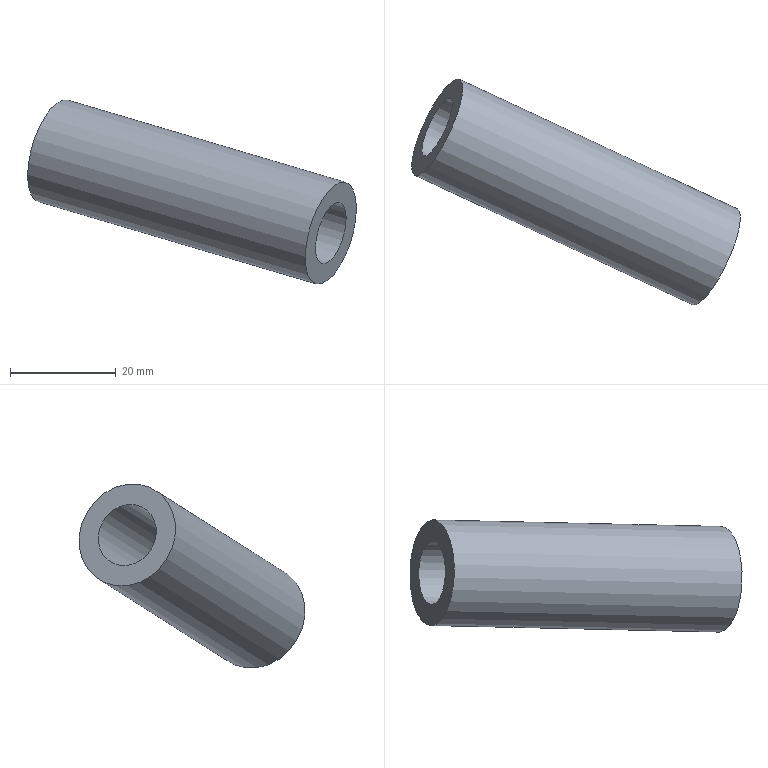Part | NX | features solid 2 | 1 solid | 4 faces | box 62.193 x 42.751 x 34.848 mm | volume 12064 mm3 | cylinder 2 | plane 2 | commonest cylinder face diameters 12 x1 20 x1
STEP:
#1=CARTESIAN_POINT('',(-896.209,778.382,-91.518));
#2=VERTEX_POINT('',#1);
#3=CARTESIAN_POINT('',(-891.983,787.445,-91.518));
#4=DIRECTION('',(-0.8754,0.4082,0.2588));
#5=DIRECTION('',(-0.4226,-0.9063,-0.000000003));
#6=AXIS2_PLACEMENT_3D('',#3,#4,#5);
#7=CIRCLE('',#6,10.);
#8=EDGE_CURVE('',#2,#2,#7,.F.);
#9=ORIENTED_EDGE('',*,*,#8,.T.);
#10=EDGE_LOOP('',(#9));
#11=FACE_BOUND('',#10,.T.);
#12=CARTESIAN_POINT('',(-843.684,753.889,-107.047));
#13=VERTEX_POINT('',#12);
#14=CARTESIAN_POINT('',(-839.458,762.952,-107.047));
#15=DIRECTION('',(-0.8754,0.4082,0.2588));
#16=DIRECTION('',(-0.4226,-0.9063,-0.000000003));
#17=AXIS2_PLACEMENT_3D('',#14,#15,#16);
#18=CIRCLE('',#17,10.);
#19=EDGE_CURVE('',#13,#13,#18,.F.);
#20=ORIENTED_EDGE('',*,*,#19,.F.);
#21=EDGE_LOOP('',(#20));
#22=FACE_BOUND('',#21,.T.);
#23=CARTESIAN_POINT('',(-839.458,762.952,-107.047));
#24=DIRECTION('',(-0.8754,0.4082,0.2588));
#25=DIRECTION('',(-0.4226,-0.9063,-0.000000003));
#26=AXIS2_PLACEMENT_3D('',#23,#24,#25);
#27=CYLINDRICAL_SURFACE('',#26,10.);
#28=ADVANCED_FACE('',(#11,#22),#27,.T.);
#29=ORIENTED_EDGE('',*,*,#19,.T.);
#30=EDGE_LOOP('',(#29));
#31=FACE_BOUND('',#30,.T.);
#32=CARTESIAN_POINT('',(-841.993,757.514,-107.047));
#33=VERTEX_POINT('',#32);
#34=CARTESIAN_POINT('',(-839.458,762.952,-107.047));
#35=DIRECTION('',(0.8754,-0.4082,-0.2588));
#36=DIRECTION('',(-0.4226,-0.9063,-0.000000003));
#37=AXIS2_PLACEMENT_3D('',#34,#35,#36);
#38=CIRCLE('',#37,6.);
#39=EDGE_CURVE('',#33,#33,#38,.T.);
#40=ORIENTED_EDGE('',*,*,#39,.F.);
#41=EDGE_LOOP('',(#40));
#42=FACE_BOUND('',#41,.T.);
#43=CARTESIAN_POINT('',(-839.458,762.952,-107.047));
#44=DIRECTION('',(-0.8754,0.4082,0.2588));
#45=DIRECTION('',(-0.4226,-0.9063,-0.000000003));
#46=AXIS2_PLACEMENT_3D('',#43,#44,#45);
#47=PLANE('',#46);
#48=ADVANCED_FACE('',(#31,#42),#47,.F.);
#49=ORIENTED_EDGE('',*,*,#8,.F.);
#50=EDGE_LOOP('',(#49));
#51=FACE_BOUND('',#50,.T.);
#52=CARTESIAN_POINT('',(-894.519,782.007,-91.518));
#53=VERTEX_POINT('',#52);
#54=CARTESIAN_POINT('',(-891.983,787.445,-91.518));
#55=DIRECTION('',(-0.8754,0.4082,0.2588));
#56=DIRECTION('',(-0.4226,-0.9063,-0.000000003));
#57=AXIS2_PLACEMENT_3D('',#54,#55,#56);
#58=CIRCLE('',#57,6.);
#59=EDGE_CURVE('',#53,#53,#58,.F.);
#60=ORIENTED_EDGE('',*,*,#59,.T.);
#61=EDGE_LOOP('',(#60));
#62=FACE_BOUND('',#61,.T.);
#63=CARTESIAN_POINT('',(-891.983,787.445,-91.518));
#64=DIRECTION('',(-0.8754,0.4082,0.2588));
#65=DIRECTION('',(-0.4226,-0.9063,-0.000000003));
#66=AXIS2_PLACEMENT_3D('',#63,#64,#65);
#67=PLANE('',#66);
#68=ADVANCED_FACE('',(#51,#62),#67,.T.);
#69=ORIENTED_EDGE('',*,*,#59,.F.);
#70=EDGE_LOOP('',(#69));
#71=FACE_BOUND('',#70,.T.);
#72=ORIENTED_EDGE('',*,*,#39,.T.);
#73=EDGE_LOOP('',(#72));
#74=FACE_BOUND('',#73,.T.);
#75=CARTESIAN_POINT('',(-839.458,762.952,-107.047));
#76=DIRECTION('',(-0.8754,0.4082,0.2588));
#77=DIRECTION('',(-0.4226,-0.9063,-0.000000003));
#78=AXIS2_PLACEMENT_3D('',#75,#76,#77);
#79=CYLINDRICAL_SURFACE('',#78,6.);
#80=ADVANCED_FACE('',(#71,#74),#79,.F.);
#81=CLOSED_SHELL('',(#28,#48,#68,#80));
#82=MANIFOLD_SOLID_BREP('',#81);
#83=(LENGTH_UNIT()NAMED_UNIT(*)SI_UNIT(.MILLI.,.METRE.));
#84=UNCERTAINTY_MEASURE_WITH_UNIT(LENGTH_MEASURE(0.00001),#83,'','');
#85=(NAMED_UNIT(*)PLANE_ANGLE_UNIT()SI_UNIT($,.RADIAN.));
#86=(NAMED_UNIT(*)SI_UNIT($,.STERADIAN.)SOLID_ANGLE_UNIT());
#87=(GEOMETRIC_REPRESENTATION_CONTEXT(3)GLOBAL_UNCERTAINTY_ASSIGNED_CONTEXT((#84))GLOBAL_UNIT_ASSIGNED_CONTEXT((#83,#85,#86))REPRESENTATION_CONTEXT('',''));
#88=ADVANCED_BREP_SHAPE_REPRESENTATION('',(#82),#87);